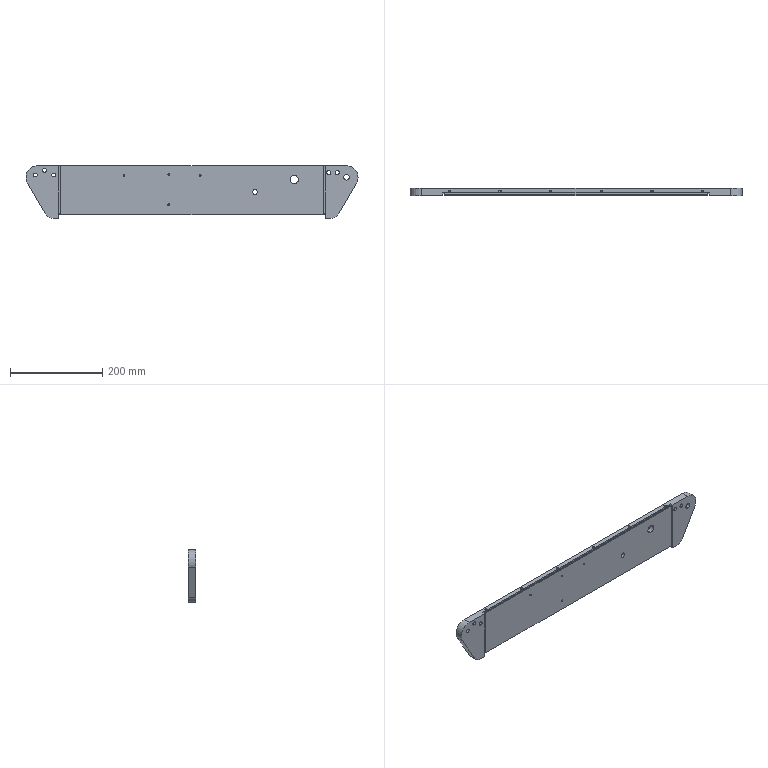Part | SolidWorks | features BaseBody 1 | 1 solid | 195 faces | box 720.1 x 16 x 114 mm | volume 1127482 mm3 | cylinder 92 | cone 66 | plane 37 | commonest cylinder face diameters 5 x28 4.2 x20 8.4 x10 2.5 x8 1 x4 8.6 x4